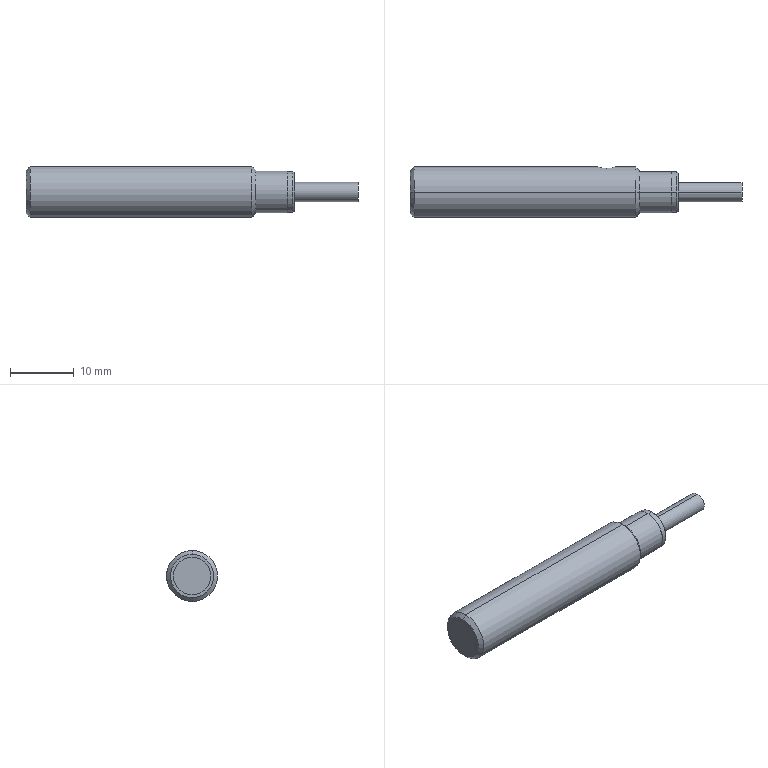Part | SolidWorks | features BaseBody 1 | 1 solid | 32 faces | box 52.05 x 8 x 8 mm | volume 2062 mm3 | cylinder 14 | plane 12 | cone 6 | commonest cylinder face diameters 3 x4 1.8 x2 5.9 x2 6.4 x2 6.5 x2 8 x2
STEP:
#1=CARTESIAN_POINT('',(30.8,3.708,-1.5));
#2=VERTEX_POINT('',#1);
#3=CARTESIAN_POINT('',(30.8,3.708,1.5));
#4=VERTEX_POINT('',#3);
#5=CARTESIAN_POINT('',(30.8,3.708,-1.5));
#6=CARTESIAN_POINT('',(30.997,3.708,-1.5));
#7=CARTESIAN_POINT('',(31.196,3.725,-1.46));
#8=CARTESIAN_POINT('',(31.467,3.767,-1.347));
#9=CARTESIAN_POINT('',(31.555,3.783,-1.3));
#10=CARTESIAN_POINT('',(31.717,3.819,-1.191));
#11=CARTESIAN_POINT('',(31.792,3.838,-1.13));
#12=CARTESIAN_POINT('',(31.999,3.895,-0.9226));
#13=CARTESIAN_POINT('',(32.109,3.932,-0.7596));
#14=CARTESIAN_POINT('',(32.223,3.972,-0.4853));
#15=CARTESIAN_POINT('',(32.251,3.982,-0.3914));
#16=CARTESIAN_POINT('',(32.29,3.996,-0.1986));
#17=CARTESIAN_POINT('',(32.3,4.,-0.09852));
#18=CARTESIAN_POINT('',(32.3,4.,0.09993));
#19=CARTESIAN_POINT('',(32.29,3.996,0.198));
#20=CARTESIAN_POINT('',(32.251,3.982,0.392));
#21=CARTESIAN_POINT('',(32.222,3.971,0.4877));
#22=CARTESIAN_POINT('',(32.109,3.932,0.7588));
#23=CARTESIAN_POINT('',(31.997,3.894,0.9245));
#24=CARTESIAN_POINT('',(31.791,3.838,1.13));
#25=CARTESIAN_POINT('',(31.715,3.818,1.193));
#26=CARTESIAN_POINT('',(31.553,3.783,1.301));
#27=CARTESIAN_POINT('',(31.467,3.767,1.347));
#28=CARTESIAN_POINT('',(31.286,3.739,1.423));
#29=CARTESIAN_POINT('',(31.19,3.727,1.452));
#30=CARTESIAN_POINT('',(30.997,3.712,1.49));
#31=CARTESIAN_POINT('',(30.9,3.708,1.5));
#32=CARTESIAN_POINT('',(30.8,3.708,1.5));
#33=B_SPLINE_CURVE_WITH_KNOTS('',3,(#5,#6,#7,#8,#9,#10,#11,#12,#13,#14,#15,#16,#17,#18,#19,#20,#21,#22,#23,#24,#25,#26,#27,#28,#29,#30,#31,#32),.UNSPECIFIED.,.F.,.F.,(4,2,2,2,2,2,2,2,2,2,2,2,2,4),(0.004683,0.005275,0.005571,0.005866,0.006458,0.006754,0.007049,0.007345,0.007641,0.008233,0.008528,0.008824,0.00912,0.009416),.UNSPECIFIED.);
#34=EDGE_CURVE('',#2,#4,#33,.T.);
#35=ORIENTED_EDGE('',*,*,#34,.T.);
#36=CARTESIAN_POINT('',(30.8,3.708,1.5));
#37=CARTESIAN_POINT('',(30.601,3.708,1.5));
#38=CARTESIAN_POINT('',(30.404,3.725,1.46));
#39=CARTESIAN_POINT('',(30.131,3.767,1.346));
#40=CARTESIAN_POINT('',(30.046,3.783,1.3));
#41=CARTESIAN_POINT('',(29.884,3.819,1.192));
#42=CARTESIAN_POINT('',(29.808,3.838,1.129));
#43=CARTESIAN_POINT('',(29.602,3.895,0.9231));
#44=CARTESIAN_POINT('',(29.491,3.932,0.7572));
#45=CARTESIAN_POINT('',(29.34,3.984,0.3969));
#46=CARTESIAN_POINT('',(29.3,4.,0.1979));
#47=CARTESIAN_POINT('',(29.3,4.,-0.0981));
#48=CARTESIAN_POINT('',(29.31,3.996,-0.1984));
#49=CARTESIAN_POINT('',(29.349,3.982,-0.3921));
#50=CARTESIAN_POINT('',(29.378,3.971,-0.486));
#51=CARTESIAN_POINT('',(29.491,3.932,-0.759));
#52=CARTESIAN_POINT('',(29.602,3.895,-0.9233));
#53=CARTESIAN_POINT('',(29.809,3.838,-1.13));
#54=CARTESIAN_POINT('',(29.884,3.819,-1.192));
#55=CARTESIAN_POINT('',(30.046,3.783,-1.3));
#56=CARTESIAN_POINT('',(30.133,3.767,-1.347));
#57=CARTESIAN_POINT('',(30.314,3.739,-1.422));
#58=CARTESIAN_POINT('',(30.407,3.728,-1.451));
#59=CARTESIAN_POINT('',(30.601,3.712,-1.49));
#60=CARTESIAN_POINT('',(30.701,3.708,-1.5));
#61=CARTESIAN_POINT('',(30.8,3.708,-1.5));
#62=B_SPLINE_CURVE_WITH_KNOTS('',3,(#36,#37,#38,#39,#40,#41,#42,#43,#44,#45,#46,#47,#48,#49,#50,#51,#52,#53,#54,#55,#56,#57,#58,#59,#60,#61),.UNSPECIFIED.,.F.,.F.,(4,2,2,2,2,2,2,2,2,2,2,2,4),(0.009416,0.01001,0.0103,0.0106,0.01119,0.01178,0.01208,0.01237,0.01296,0.01326,0.01356,0.01385,0.01415),.UNSPECIFIED.);
#63=EDGE_CURVE('',#4,#2,#62,.T.);
#64=ORIENTED_EDGE('',*,*,#63,.T.);
#65=EDGE_LOOP('',(#35,#64));
#66=FACE_BOUND('',#65,.T.);
#67=CARTESIAN_POINT('',(35.386,0.,4.));
#68=VERTEX_POINT('',#67);
#69=CARTESIAN_POINT('',(35.386,0.,-4.));
#70=VERTEX_POINT('',#69);
#71=CARTESIAN_POINT('',(35.386,0.,0.));
#72=DIRECTION('',(-1.,0.,0.));
#73=DIRECTION('',(0.,0.,1.));
#74=AXIS2_PLACEMENT_3D('',#71,#72,#73);
#75=CIRCLE('',#74,4.);
#76=EDGE_CURVE('',#68,#70,#75,.T.);
#77=ORIENTED_EDGE('',*,*,#76,.T.);
#78=CARTESIAN_POINT('',(0.6635,0.,-4.));
#79=VERTEX_POINT('',#78);
#80=CARTESIAN_POINT('',(52.05,0.,-4.));
#81=DIRECTION('',(-1.,0.,0.));
#82=VECTOR('',#81,1000.);
#83=LINE('',#80,#82);
#84=EDGE_CURVE('',#70,#79,#83,.T.);
#85=ORIENTED_EDGE('',*,*,#84,.T.);
#86=CARTESIAN_POINT('',(0.6635,0.,4.));
#87=VERTEX_POINT('',#86);
#88=CARTESIAN_POINT('',(0.6635,0.,0.));
#89=DIRECTION('',(1.,0.,0.));
#90=DIRECTION('',(0.,0.,1.));
#91=AXIS2_PLACEMENT_3D('',#88,#89,#90);
#92=CIRCLE('',#91,4.);
#93=EDGE_CURVE('',#79,#87,#92,.T.);
#94=ORIENTED_EDGE('',*,*,#93,.T.);
#95=CARTESIAN_POINT('',(52.05,0.,4.));
#96=DIRECTION('',(-1.,0.,0.));
#97=VECTOR('',#96,1000.);
#98=LINE('',#95,#97);
#99=EDGE_CURVE('',#68,#87,#98,.T.);
#100=ORIENTED_EDGE('',*,*,#99,.F.);
#101=EDGE_LOOP('',(#77,#85,#94,#100));
#102=FACE_OUTER_BOUND('',#101,.T.);
#103=CARTESIAN_POINT('',(52.05,0.,0.));
#104=DIRECTION('',(-1.,0.,0.));
#105=DIRECTION('',(0.,0.,1.));
#106=AXIS2_PLACEMENT_3D('',#103,#104,#105);
#107=CYLINDRICAL_SURFACE('',#106,4.);
#108=ADVANCED_FACE('',(#66,#102),#107,.T.);
#109=CARTESIAN_POINT('',(0.05,0.,-3.386));
#110=VERTEX_POINT('',#109);
#111=CARTESIAN_POINT('',(0.05,0.,3.386));
#112=VERTEX_POINT('',#111);
#113=CARTESIAN_POINT('',(0.05,0.,0.));
#114=DIRECTION('',(1.,0.,0.));
#115=DIRECTION('',(0.,0.,-1.));
#116=AXIS2_PLACEMENT_3D('',#113,#114,#115);
#117=CIRCLE('',#116,3.386);
#118=EDGE_CURVE('',#110,#112,#117,.T.);
#119=ORIENTED_EDGE('',*,*,#118,.T.);
#120=CARTESIAN_POINT('',(0.6635,0.,4.));
#121=DIRECTION('',(0.7071,0.,0.7071));
#122=VECTOR('',#121,1000.);
#123=LINE('',#120,#122);
#124=EDGE_CURVE('',#112,#87,#123,.T.);
#125=ORIENTED_EDGE('',*,*,#124,.T.);
#126=ORIENTED_EDGE('',*,*,#93,.F.);
#127=CARTESIAN_POINT('',(0.6635,0.,-4.));
#128=DIRECTION('',(0.7071,0.,-0.7071));
#129=VECTOR('',#128,1000.);
#130=LINE('',#127,#129);
#131=EDGE_CURVE('',#110,#79,#130,.T.);
#132=ORIENTED_EDGE('',*,*,#131,.F.);
#133=EDGE_LOOP('',(#119,#125,#126,#132));
#134=FACE_OUTER_BOUND('',#133,.T.);
#135=CARTESIAN_POINT('',(0.6635,0.,0.));
#136=DIRECTION('',(1.,0.,0.));
#137=DIRECTION('',(0.,0.,-1.));
#138=AXIS2_PLACEMENT_3D('',#135,#136,#137);
#139=CONICAL_SURFACE('',#138,4.,0.7854);
#140=ADVANCED_FACE('',(#134),#139,.T.);
#141=ORIENTED_EDGE('',*,*,#63,.F.);
#142=CARTESIAN_POINT('',(30.8,2.75,1.5));
#143=VERTEX_POINT('',#142);
#144=CARTESIAN_POINT('',(30.8,2.75,1.5));
#145=DIRECTION('',(0.,-1.,0.));
#146=VECTOR('',#145,1000.);
#147=LINE('',#144,#146);
#148=EDGE_CURVE('',#4,#143,#147,.T.);
#149=ORIENTED_EDGE('',*,*,#148,.T.);
#150=CARTESIAN_POINT('',(30.8,2.75,-1.5));
#151=VERTEX_POINT('',#150);
#152=CARTESIAN_POINT('',(30.8,2.75,0.));
#153=DIRECTION('',(0.,1.,0.));
#154=DIRECTION('',(0.,0.,-1.));
#155=AXIS2_PLACEMENT_3D('',#152,#153,#154);
#156=CIRCLE('',#155,1.5);
#157=EDGE_CURVE('',#151,#143,#156,.T.);
#158=ORIENTED_EDGE('',*,*,#157,.F.);
#159=CARTESIAN_POINT('',(30.8,2.75,-1.5));
#160=DIRECTION('',(0.,-1.,0.));
#161=VECTOR('',#160,1000.);
#162=LINE('',#159,#161);
#163=EDGE_CURVE('',#2,#151,#162,.T.);
#164=ORIENTED_EDGE('',*,*,#163,.F.);
#165=EDGE_LOOP('',(#141,#149,#158,#164));
#166=FACE_OUTER_BOUND('',#165,.T.);
#167=CARTESIAN_POINT('',(30.8,2.75,0.));
#168=DIRECTION('',(0.,-1.,0.));
#169=DIRECTION('',(0.,0.,-1.));
#170=AXIS2_PLACEMENT_3D('',#167,#168,#169);
#171=CYLINDRICAL_SURFACE('',#170,1.5);
#172=ADVANCED_FACE('',(#166),#171,.F.);
#173=CARTESIAN_POINT('',(36.,0.,3.387));
#174=VERTEX_POINT('',#173);
#175=CARTESIAN_POINT('',(36.,0.,-3.387));
#176=VERTEX_POINT('',#175);
#177=CARTESIAN_POINT('',(36.,0.,0.));
#178=DIRECTION('',(-1.,0.,0.));
#179=DIRECTION('',(0.,0.,1.));
#180=AXIS2_PLACEMENT_3D('',#177,#178,#179);
#181=CIRCLE('',#180,3.387);
#182=EDGE_CURVE('',#174,#176,#181,.T.);
#183=ORIENTED_EDGE('',*,*,#182,.T.);
#184=CARTESIAN_POINT('',(35.387,0.,-4.));
#185=DIRECTION('',(-0.7071,0.,-0.7071));
#186=VECTOR('',#185,1000.);
#187=LINE('',#184,#186);
#188=EDGE_CURVE('',#176,#70,#187,.T.);
#189=ORIENTED_EDGE('',*,*,#188,.T.);
#190=ORIENTED_EDGE('',*,*,#76,.F.);
#191=CARTESIAN_POINT('',(35.387,0.,4.));
#192=DIRECTION('',(-0.7071,0.,0.7071));
#193=VECTOR('',#192,1000.);
#194=LINE('',#191,#193);
#195=EDGE_CURVE('',#174,#68,#194,.T.);
#196=ORIENTED_EDGE('',*,*,#195,.F.);
#197=EDGE_LOOP('',(#183,#189,#190,#196));
#198=FACE_OUTER_BOUND('',#197,.T.);
#199=CARTESIAN_POINT('',(35.387,0.,0.));
#200=DIRECTION('',(-1.,0.,0.));
#201=DIRECTION('',(0.,0.,1.));
#202=AXIS2_PLACEMENT_3D('',#199,#200,#201);
#203=CONICAL_SURFACE('',#202,4.,0.7854);
#204=ADVANCED_FACE('',(#198),#203,.T.);
#205=CARTESIAN_POINT('',(0.05,0.,2.95));
#206=VERTEX_POINT('',#205);
#207=CARTESIAN_POINT('',(0.05,0.,-2.95));
#208=VERTEX_POINT('',#207);
#209=CARTESIAN_POINT('',(0.05,0.,0.));
#210=DIRECTION('',(-1.,0.,0.));
#211=DIRECTION('',(0.,0.,1.));
#212=AXIS2_PLACEMENT_3D('',#209,#210,#211);
#213=CIRCLE('',#212,2.95);
#214=EDGE_CURVE('',#206,#208,#213,.T.);
#215=ORIENTED_EDGE('',*,*,#214,.T.);
#216=CARTESIAN_POINT('',(0.,0.,-2.95));
#217=VERTEX_POINT('',#216);
#218=CARTESIAN_POINT('',(52.05,0.,-2.95));
#219=DIRECTION('',(-1.,0.,0.));
#220=VECTOR('',#219,1000.);
#221=LINE('',#218,#220);
#222=EDGE_CURVE('',#208,#217,#221,.T.);
#223=ORIENTED_EDGE('',*,*,#222,.T.);
#224=CARTESIAN_POINT('',(0.,0.,2.95));
#225=VERTEX_POINT('',#224);
#226=CARTESIAN_POINT('',(0.,0.,0.));
#227=DIRECTION('',(1.,0.,0.));
#228=DIRECTION('',(0.,0.,1.));
#229=AXIS2_PLACEMENT_3D('',#226,#227,#228);
#230=CIRCLE('',#229,2.95);
#231=EDGE_CURVE('',#217,#225,#230,.T.);
#232=ORIENTED_EDGE('',*,*,#231,.T.);
#233=CARTESIAN_POINT('',(52.05,0.,2.95));
#234=DIRECTION('',(-1.,0.,0.));
#235=VECTOR('',#234,1000.);
#236=LINE('',#233,#235);
#237=EDGE_CURVE('',#206,#225,#236,.T.);
#238=ORIENTED_EDGE('',*,*,#237,.F.);
#239=EDGE_LOOP('',(#215,#223,#232,#238));
#240=FACE_OUTER_BOUND('',#239,.T.);
#241=CARTESIAN_POINT('',(52.05,0.,0.));
#242=DIRECTION('',(-1.,0.,0.));
#243=DIRECTION('',(0.,0.,1.));
#244=AXIS2_PLACEMENT_3D('',#241,#242,#243);
#245=CYLINDRICAL_SURFACE('',#244,2.95);
#246=ADVANCED_FACE('',(#240),#245,.T.);
#247=CARTESIAN_POINT('',(30.8,2.9,0.9));
#248=VERTEX_POINT('',#247);
#249=CARTESIAN_POINT('',(31.05,2.9,0.8646));
#250=VERTEX_POINT('',#249);
#251=CARTESIAN_POINT('',(30.8,2.9,0.));
#252=DIRECTION('',(0.,1.,0.));
#253=DIRECTION('',(0.,0.,-1.));
#254=AXIS2_PLACEMENT_3D('',#251,#252,#253);
#255=CIRCLE('',#254,0.9);
#256=EDGE_CURVE('',#248,#250,#255,.T.);
#257=ORIENTED_EDGE('',*,*,#256,.F.);
#258=CARTESIAN_POINT('',(30.8,2.75,0.9));
#259=VERTEX_POINT('',#258);
#260=CARTESIAN_POINT('',(30.8,2.55,0.9));
#261=DIRECTION('',(0.,-1.,0.));
#262=VECTOR('',#261,1000.);
#263=LINE('',#260,#262);
#264=EDGE_CURVE('',#248,#259,#263,.T.);
#265=ORIENTED_EDGE('',*,*,#264,.T.);
#266=CARTESIAN_POINT('',(30.8,2.75,-0.9));
#267=VERTEX_POINT('',#266);
#268=CARTESIAN_POINT('',(30.8,2.75,0.));
#269=DIRECTION('',(0.,-1.,0.));
#270=DIRECTION('',(0.,0.,-1.));
#271=AXIS2_PLACEMENT_3D('',#268,#269,#270);
#272=CIRCLE('',#271,0.9);
#273=EDGE_CURVE('',#267,#259,#272,.T.);
#274=ORIENTED_EDGE('',*,*,#273,.F.);
#275=CARTESIAN_POINT('',(30.8,2.9,-0.9));
#276=VERTEX_POINT('',#275);
#277=CARTESIAN_POINT('',(30.8,2.55,-0.9));
#278=DIRECTION('',(0.,-1.,0.));
#279=VECTOR('',#278,1000.);
#280=LINE('',#277,#279);
#281=EDGE_CURVE('',#276,#267,#280,.T.);
#282=ORIENTED_EDGE('',*,*,#281,.F.);
#283=CARTESIAN_POINT('',(31.05,2.9,-0.8646));
#284=VERTEX_POINT('',#283);
#285=CARTESIAN_POINT('',(30.8,2.9,0.));
#286=DIRECTION('',(0.,1.,0.));
#287=DIRECTION('',(0.,0.,-1.));
#288=AXIS2_PLACEMENT_3D('',#285,#286,#287);
#289=CIRCLE('',#288,0.9);
#290=EDGE_CURVE('',#284,#276,#289,.T.);
#291=ORIENTED_EDGE('',*,*,#290,.F.);
#292=CARTESIAN_POINT('',(31.05,3.05,-0.8646));
#293=VERTEX_POINT('',#292);
#294=CARTESIAN_POINT('',(31.05,2.9,-0.8646));
#295=DIRECTION('',(0.,1.,0.));
#296=VECTOR('',#295,1000.);
#297=LINE('',#294,#296);
#298=EDGE_CURVE('',#284,#293,#297,.T.);
#299=ORIENTED_EDGE('',*,*,#298,.T.);
#300=CARTESIAN_POINT('',(31.05,3.05,0.8646));
#301=VERTEX_POINT('',#300);
#302=CARTESIAN_POINT('',(30.8,3.05,0.));
#303=DIRECTION('',(0.,-1.,0.));
#304=DIRECTION('',(0.,0.,-1.));
#305=AXIS2_PLACEMENT_3D('',#302,#303,#304);
#306=CIRCLE('',#305,0.9);
#307=EDGE_CURVE('',#293,#301,#306,.T.);
#308=ORIENTED_EDGE('',*,*,#307,.T.);
#309=CARTESIAN_POINT('',(31.05,2.9,0.8646));
#310=DIRECTION('',(0.,-1.,0.));
#311=VECTOR('',#310,1000.);
#312=LINE('',#309,#311);
#313=EDGE_CURVE('',#301,#250,#312,.T.);
#314=ORIENTED_EDGE('',*,*,#313,.T.);
#315=EDGE_LOOP('',(#257,#265,#274,#282,#291,#299,#308,#314));
#316=FACE_OUTER_BOUND('',#315,.T.);
#317=CARTESIAN_POINT('',(30.8,2.55,0.));
#318=DIRECTION('',(0.,-1.,0.));
#319=DIRECTION('',(0.,0.,-1.));
#320=AXIS2_PLACEMENT_3D('',#317,#318,#319);
#321=CYLINDRICAL_SURFACE('',#320,0.9);
#322=ADVANCED_FACE('',(#316),#321,.T.);
#323=CARTESIAN_POINT('',(41.05,0.,3.25));
#324=VERTEX_POINT('',#323);
#325=CARTESIAN_POINT('',(41.05,0.,-3.25));
#326=VERTEX_POINT('',#325);
#327=CARTESIAN_POINT('',(41.05,0.,0.));
#328=DIRECTION('',(-1.,0.,0.));
#329=DIRECTION('',(0.,0.,1.));
#330=AXIS2_PLACEMENT_3D('',#327,#328,#329);
#331=CIRCLE('',#330,3.25);
#332=EDGE_CURVE('',#324,#326,#331,.T.);
#333=ORIENTED_EDGE('',*,*,#332,.T.);
#334=CARTESIAN_POINT('',(36.,0.,-3.25));
#335=VERTEX_POINT('',#334);
#336=CARTESIAN_POINT('',(52.05,0.,-3.25));
#337=DIRECTION('',(-1.,0.,0.));
#338=VECTOR('',#337,1000.);
#339=LINE('',#336,#338);
#340=EDGE_CURVE('',#326,#335,#339,.T.);
#341=ORIENTED_EDGE('',*,*,#340,.T.);
#342=CARTESIAN_POINT('',(36.,0.,3.25));
#343=VERTEX_POINT('',#342);
#344=CARTESIAN_POINT('',(36.,0.,0.));
#345=DIRECTION('',(1.,0.,0.));
#346=DIRECTION('',(0.,0.,1.));
#347=AXIS2_PLACEMENT_3D('',#344,#345,#346);
#348=CIRCLE('',#347,3.25);
#349=EDGE_CURVE('',#335,#343,#348,.T.);
#350=ORIENTED_EDGE('',*,*,#349,.T.);
#351=CARTESIAN_POINT('',(52.05,0.,3.25));
#352=DIRECTION('',(-1.,0.,0.));
#353=VECTOR('',#352,1000.);
#354=LINE('',#351,#353);
#355=EDGE_CURVE('',#324,#343,#354,.T.);
#356=ORIENTED_EDGE('',*,*,#355,.F.);
#357=EDGE_LOOP('',(#333,#341,#350,#356));
#358=FACE_OUTER_BOUND('',#357,.T.);
#359=CARTESIAN_POINT('',(52.05,0.,0.));
#360=DIRECTION('',(-1.,0.,0.));
#361=DIRECTION('',(0.,0.,1.));
#362=AXIS2_PLACEMENT_3D('',#359,#360,#361);
#363=CYLINDRICAL_SURFACE('',#362,3.25);
#364=ADVANCED_FACE('',(#358),#363,.T.);
#365=CARTESIAN_POINT('',(41.85,0.,3.2));
#366=VERTEX_POINT('',#365);
#367=CARTESIAN_POINT('',(41.85,0.,-3.2));
#368=VERTEX_POINT('',#367);
#369=CARTESIAN_POINT('',(41.85,0.,0.));
#370=DIRECTION('',(-1.,0.,0.));
#371=DIRECTION('',(0.,0.,1.));
#372=AXIS2_PLACEMENT_3D('',#369,#370,#371);
#373=CIRCLE('',#372,3.2);
#374=EDGE_CURVE('',#366,#368,#373,.T.);
#375=ORIENTED_EDGE('',*,*,#374,.T.);
#376=CARTESIAN_POINT('',(41.05,0.,-3.2));
#377=VERTEX_POINT('',#376);
#378=CARTESIAN_POINT('',(52.05,0.,-3.2));
#379=DIRECTION('',(-1.,0.,0.));
#380=VECTOR('',#379,1000.);
#381=LINE('',#378,#380);
#382=EDGE_CURVE('',#368,#377,#381,.T.);
#383=ORIENTED_EDGE('',*,*,#382,.T.);
#384=CARTESIAN_POINT('',(41.05,0.,3.2));
#385=VERTEX_POINT('',#384);
#386=CARTESIAN_POINT('',(41.05,0.,0.));
#387=DIRECTION('',(1.,0.,0.));
#388=DIRECTION('',(0.,0.,1.));
#389=AXIS2_PLACEMENT_3D('',#386,#387,#388);
#390=CIRCLE('',#389,3.2);
#391=EDGE_CURVE('',#377,#385,#390,.T.);
#392=ORIENTED_EDGE('',*,*,#391,.T.);
#393=CARTESIAN_POINT('',(52.05,0.,3.2));
#394=DIRECTION('',(-1.,0.,0.));
#395=VECTOR('',#394,1000.);
#396=LINE('',#393,#395);
#397=EDGE_CURVE('',#366,#385,#396,.T.);
#398=ORIENTED_EDGE('',*,*,#397,.F.);
#399=EDGE_LOOP('',(#375,#383,#392,#398));
#400=FACE_OUTER_BOUND('',#399,.T.);
#401=CARTESIAN_POINT('',(52.05,0.,0.));
#402=DIRECTION('',(-1.,0.,0.));
#403=DIRECTION('',(0.,0.,1.));
#404=AXIS2_PLACEMENT_3D('',#401,#402,#403);
#405=CYLINDRICAL_SURFACE('',#404,3.2);
#406=ADVANCED_FACE('',(#400),#405,.T.);
#407=CARTESIAN_POINT('',(42.05,0.,3.));
#408=VERTEX_POINT('',#407);
#409=CARTESIAN_POINT('',(42.05,0.,-3.));
#410=VERTEX_POINT('',#409);
#411=CARTESIAN_POINT('',(42.05,0.,0.));
#412=DIRECTION('',(-1.,0.,0.));
#413=DIRECTION('',(0.,0.,1.));
#414=AXIS2_PLACEMENT_3D('',#411,#412,#413);
#415=CIRCLE('',#414,3.);
#416=EDGE_CURVE('',#408,#410,#415,.T.);
#417=ORIENTED_EDGE('',*,*,#416,.T.);
#418=CARTESIAN_POINT('',(41.85,0.,-3.2));
#419=DIRECTION('',(-0.7071,0.,-0.7071));
#420=VECTOR('',#419,1000.);
#421=LINE('',#418,#420);
#422=EDGE_CURVE('',#410,#368,#421,.T.);
#423=ORIENTED_EDGE('',*,*,#422,.T.);
#424=ORIENTED_EDGE('',*,*,#374,.F.);
#425=CARTESIAN_POINT('',(41.85,0.,3.2));
#426=DIRECTION('',(-0.7071,0.,0.7071));
#427=VECTOR('',#426,1000.);
#428=LINE('',#425,#427);
#429=EDGE_CURVE('',#408,#366,#428,.T.);
#430=ORIENTED_EDGE('',*,*,#429,.F.);
#431=EDGE_LOOP('',(#417,#423,#424,#430));
#432=FACE_OUTER_BOUND('',#431,.T.);
#433=CARTESIAN_POINT('',(41.85,0.,0.));
#434=DIRECTION('',(-1.,0.,0.));
#435=DIRECTION('',(0.,0.,1.));
#436=AXIS2_PLACEMENT_3D('',#433,#434,#435);
#437=CONICAL_SURFACE('',#436,3.2,0.7854);
#438=ADVANCED_FACE('',(#432),#437,.T.);
#439=CARTESIAN_POINT('',(52.05,0.,1.5));
#440=VERTEX_POINT('',#439);
#441=CARTESIAN_POINT('',(52.05,0.,-1.5));
#442=VERTEX_POINT('',#441);
#443=CARTESIAN_POINT('',(52.05,0.,0.));
#444=DIRECTION('',(-1.,0.,0.));
#445=DIRECTION('',(0.,0.,1.));
#446=AXIS2_PLACEMENT_3D('',#443,#444,#445);
#447=CIRCLE('',#446,1.5);
#448=EDGE_CURVE('',#440,#442,#447,.T.);
#449=ORIENTED_EDGE('',*,*,#448,.T.);
#450=CARTESIAN_POINT('',(42.05,0.,-1.5));
#451=VERTEX_POINT('',#450);
#452=CARTESIAN_POINT('',(52.05,0.,-1.5));
#453=DIRECTION('',(-1.,0.,0.));
#454=VECTOR('',#453,1000.);
#455=LINE('',#452,#454);
#456=EDGE_CURVE('',#442,#451,#455,.T.);
#457=ORIENTED_EDGE('',*,*,#456,.T.);
#458=CARTESIAN_POINT('',(42.05,0.,1.5));
#459=VERTEX_POINT('',#458);
#460=CARTESIAN_POINT('',(42.05,0.,0.));
#461=DIRECTION('',(1.,0.,0.));
#462=DIRECTION('',(0.,0.,1.));
#463=AXIS2_PLACEMENT_3D('',#460,#461,#462);
#464=CIRCLE('',#463,1.5);
#465=EDGE_CURVE('',#451,#459,#464,.T.);
#466=ORIENTED_EDGE('',*,*,#465,.T.);
#467=CARTESIAN_POINT('',(52.05,0.,1.5));
#468=DIRECTION('',(-1.,0.,0.));
#469=VECTOR('',#468,1000.);
#470=LINE('',#467,#469);
#471=EDGE_CURVE('',#440,#459,#470,.T.);
#472=ORIENTED_EDGE('',*,*,#471,.F.);
#473=EDGE_LOOP('',(#449,#457,#466,#472));
#474=FACE_OUTER_BOUND('',#473,.T.);
#475=CARTESIAN_POINT('',(52.05,0.,0.));
#476=DIRECTION('',(-1.,0.,0.));
#477=DIRECTION('',(0.,0.,1.));
#478=AXIS2_PLACEMENT_3D('',#475,#476,#477);
#479=CYLINDRICAL_SURFACE('',#478,1.5);
#480=ADVANCED_FACE('',(#474),#479,.T.);
#481=ORIENTED_EDGE('',*,*,#84,.F.);
#482=CARTESIAN_POINT('',(35.386,0.,0.));
#483=DIRECTION('',(-1.,0.,0.));
#484=DIRECTION('',(0.,0.,1.));
#485=AXIS2_PLACEMENT_3D('',#482,#483,#484);
#486=CIRCLE('',#485,4.);
#487=EDGE_CURVE('',#70,#68,#486,.T.);
#488=ORIENTED_EDGE('',*,*,#487,.T.);
#489=ORIENTED_EDGE('',*,*,#99,.T.);
#490=CARTESIAN_POINT('',(0.6635,0.,0.));
#491=DIRECTION('',(1.,0.,0.));
#492=DIRECTION('',(0.,0.,1.));
#493=AXIS2_PLACEMENT_3D('',#490,#491,#492);
#494=CIRCLE('',#493,4.);
#495=EDGE_CURVE('',#87,#79,#494,.T.);
#496=ORIENTED_EDGE('',*,*,#495,.T.);
#497=EDGE_LOOP('',(#481,#488,#489,#496));
#498=FACE_OUTER_BOUND('',#497,.T.);
#499=CARTESIAN_POINT('',(52.05,0.,0.));
#500=DIRECTION('',(-1.,0.,0.));
#501=DIRECTION('',(0.,0.,1.));
#502=AXIS2_PLACEMENT_3D('',#499,#500,#501);
#503=CYLINDRICAL_SURFACE('',#502,4.);
#504=ADVANCED_FACE('',(#498),#503,.T.);
#505=ORIENTED_EDGE('',*,*,#124,.F.);
#506=CARTESIAN_POINT('',(0.05,0.,0.));
#507=DIRECTION('',(1.,0.,0.));
#508=DIRECTION('',(0.,0.,-1.));
#509=AXIS2_PLACEMENT_3D('',#506,#507,#508);
#510=CIRCLE('',#509,3.386);
#511=EDGE_CURVE('',#112,#110,#510,.T.);
#512=ORIENTED_EDGE('',*,*,#511,.T.);
#513=ORIENTED_EDGE('',*,*,#131,.T.);
#514=ORIENTED_EDGE('',*,*,#495,.F.);
#515=EDGE_LOOP('',(#505,#512,#513,#514));
#516=FACE_OUTER_BOUND('',#515,.T.);
#517=CARTESIAN_POINT('',(0.6635,0.,0.));
#518=DIRECTION('',(1.,0.,0.));
#519=DIRECTION('',(0.,0.,-1.));
#520=AXIS2_PLACEMENT_3D('',#517,#518,#519);
#521=CONICAL_SURFACE('',#520,4.,0.7854);
#522=ADVANCED_FACE('',(#516),#521,.T.);
#523=ORIENTED_EDGE('',*,*,#148,.F.);
#524=ORIENTED_EDGE('',*,*,#34,.F.);
#525=ORIENTED_EDGE('',*,*,#163,.T.);
#526=CARTESIAN_POINT('',(30.8,2.75,0.));
#527=DIRECTION('',(0.,1.,0.));
#528=DIRECTION('',(0.,0.,-1.));
#529=AXIS2_PLACEMENT_3D('',#526,#527,#528);
#530=CIRCLE('',#529,1.5);
#531=EDGE_CURVE('',#143,#151,#530,.T.);
#532=ORIENTED_EDGE('',*,*,#531,.F.);
#533=EDGE_LOOP('',(#523,#524,#525,#532));
#534=FACE_OUTER_BOUND('',#533,.T.);
#535=CARTESIAN_POINT('',(30.8,2.75,0.));
#536=DIRECTION('',(0.,-1.,0.));
#537=DIRECTION('',(0.,0.,-1.));
#538=AXIS2_PLACEMENT_3D('',#535,#536,#537);
#539=CYLINDRICAL_SURFACE('',#538,1.5);
#540=ADVANCED_FACE('',(#534),#539,.F.);
#541=ORIENTED_EDGE('',*,*,#188,.F.);
#542=CARTESIAN_POINT('',(36.,0.,0.));
#543=DIRECTION('',(-1.,0.,0.));
#544=DIRECTION('',(0.,0.,1.));
#545=AXIS2_PLACEMENT_3D('',#542,#543,#544);
#546=CIRCLE('',#545,3.387);
#547=EDGE_CURVE('',#176,#174,#546,.T.);
#548=ORIENTED_EDGE('',*,*,#547,.T.);
#549=ORIENTED_EDGE('',*,*,#195,.T.);
#550=ORIENTED_EDGE('',*,*,#487,.F.);
#551=EDGE_LOOP('',(#541,#548,#549,#550));
#552=FACE_OUTER_BOUND('',#551,.T.);
#553=CARTESIAN_POINT('',(35.387,0.,0.));
#554=DIRECTION('',(-1.,0.,0.));
#555=DIRECTION('',(0.,0.,1.));
#556=AXIS2_PLACEMENT_3D('',#553,#554,#555);
#557=CONICAL_SURFACE('',#556,4.,0.7854);
#558=ADVANCED_FACE('',(#552),#557,.T.);
#559=ORIENTED_EDGE('',*,*,#214,.F.);
#560=CARTESIAN_POINT('',(0.05,0.,0.));
#561=DIRECTION('',(-1.,0.,0.));
#562=DIRECTION('',(0.,0.,1.));
#563=AXIS2_PLACEMENT_3D('',#560,#561,#562);
#564=CIRCLE('',#563,2.95);
#565=EDGE_CURVE('',#208,#206,#564,.T.);
#566=ORIENTED_EDGE('',*,*,#565,.F.);
#567=EDGE_LOOP('',(#559,#566));
#568=FACE_BOUND('',#567,.T.);
#569=ORIENTED_EDGE('',*,*,#118,.F.);
#570=ORIENTED_EDGE('',*,*,#511,.F.);
#571=EDGE_LOOP('',(#569,#570));
#572=FACE_OUTER_BOUND('',#571,.T.);
#573=CARTESIAN_POINT('',(0.05,2.95,0.));
#574=DIRECTION('',(1.,0.,0.));
#575=DIRECTION('',(0.,0.,-1.));
#576=AXIS2_PLACEMENT_3D('',#573,#574,#575);
#577=PLANE('',#576);
#578=ADVANCED_FACE('',(#568,#572),#577,.F.);
#579=ORIENTED_EDGE('',*,*,#157,.T.);
#580=ORIENTED_EDGE('',*,*,#531,.T.);
#581=EDGE_LOOP('',(#579,#580));
#582=FACE_OUTER_BOUND('',#581,.T.);
#583=ORIENTED_EDGE('',*,*,#273,.T.);
#584=CARTESIAN_POINT('',(30.8,2.75,0.));
#585=DIRECTION('',(0.,-1.,0.));
#586=DIRECTION('',(0.,0.,-1.));
#587=AXIS2_PLACEMENT_3D('',#584,#585,#586);
#588=CIRCLE('',#587,0.9);
#589=EDGE_CURVE('',#259,#267,#588,.T.);
#590=ORIENTED_EDGE('',*,*,#589,.T.);
#591=EDGE_LOOP('',(#583,#590));
#592=FACE_BOUND('',#591,.T.);
#593=CARTESIAN_POINT('',(30.8,2.75,0.));
#594=DIRECTION('',(0.,1.,0.));
#595=DIRECTION('',(0.,0.,1.));
#596=AXIS2_PLACEMENT_3D('',#593,#594,#595);
#597=PLANE('',#596);
#598=ADVANCED_FACE('',(#582,#592),#597,.T.);
#599=ORIENTED_EDGE('',*,*,#182,.F.);
#600=ORIENTED_EDGE('',*,*,#547,.F.);
#601=EDGE_LOOP('',(#599,#600));
#602=FACE_OUTER_BOUND('',#601,.T.);
#603=CARTESIAN_POINT('',(36.,0.,0.));
#604=DIRECTION('',(1.,0.,0.));
#605=DIRECTION('',(0.,0.,1.));
#606=AXIS2_PLACEMENT_3D('',#603,#604,#605);
#607=CIRCLE('',#606,3.25);
#608=EDGE_CURVE('',#343,#335,#607,.T.);
#609=ORIENTED_EDGE('',*,*,#608,.F.);
#610=ORIENTED_EDGE('',*,*,#349,.F.);
#611=EDGE_LOOP('',(#609,#610));
#612=FACE_BOUND('',#611,.T.);
#613=CARTESIAN_POINT('',(36.,3.386,0.));
#614=DIRECTION('',(-1.,0.,0.));
#615=DIRECTION('',(0.,0.,1.));
#616=AXIS2_PLACEMENT_3D('',#613,#614,#615);
#617=PLANE('',#616);
#618=ADVANCED_FACE('',(#602,#612),#617,.F.);
#619=ORIENTED_EDGE('',*,*,#222,.F.);
#620=ORIENTED_EDGE('',*,*,#565,.T.);
#621=ORIENTED_EDGE('',*,*,#237,.T.);
#622=CARTESIAN_POINT('',(0.,0.,0.));
#623=DIRECTION('',(1.,0.,0.));
#624=DIRECTION('',(0.,0.,1.));
#625=AXIS2_PLACEMENT_3D('',#622,#623,#624);
#626=CIRCLE('',#625,2.95);
#627=EDGE_CURVE('',#225,#217,#626,.T.);
#628=ORIENTED_EDGE('',*,*,#627,.T.);
#629=EDGE_LOOP('',(#619,#620,#621,#628));
#630=FACE_OUTER_BOUND('',#629,.T.);
#631=CARTESIAN_POINT('',(52.05,0.,0.));
#632=DIRECTION('',(-1.,0.,0.));
#633=DIRECTION('',(0.,0.,1.));
#634=AXIS2_PLACEMENT_3D('',#631,#632,#633);
#635=CYLINDRICAL_SURFACE('',#634,2.95);
#636=ADVANCED_FACE('',(#630),#635,.T.);
#637=ORIENTED_EDGE('',*,*,#264,.F.);
#638=CARTESIAN_POINT('',(30.55,2.9,0.8646));
#639=VERTEX_POINT('',#638);
#640=CARTESIAN_POINT('',(30.8,2.9,0.));
#641=DIRECTION('',(0.,1.,0.));
#642=DIRECTION('',(0.,0.,-1.));
#643=AXIS2_PLACEMENT_3D('',#640,#641,#642);
#644=CIRCLE('',#643,0.9);
#645=EDGE_CURVE('',#639,#248,#644,.T.);
#646=ORIENTED_EDGE('',*,*,#645,.F.);
#647=CARTESIAN_POINT('',(30.55,3.05,0.8646));
#648=VERTEX_POINT('',#647);
#649=CARTESIAN_POINT('',(30.55,2.9,0.8646));
#650=DIRECTION('',(0.,1.,0.));
#651=VECTOR('',#650,1000.);
#652=LINE('',#649,#651);
#653=EDGE_CURVE('',#639,#648,#652,.T.);
#654=ORIENTED_EDGE('',*,*,#653,.T.);
#655=CARTESIAN_POINT('',(30.55,3.05,-0.8646));
#656=VERTEX_POINT('',#655);
#657=CARTESIAN_POINT('',(30.8,3.05,0.));
#658=DIRECTION('',(0.,-1.,0.));
#659=DIRECTION('',(0.,0.,-1.));
#660=AXIS2_PLACEMENT_3D('',#657,#658,#659);
#661=CIRCLE('',#660,0.9);
#662=EDGE_CURVE('',#648,#656,#661,.T.);
#663=ORIENTED_EDGE('',*,*,#662,.T.);
#664=CARTESIAN_POINT('',(30.55,2.9,-0.8646));
#665=VERTEX_POINT('',#664);
#666=CARTESIAN_POINT('',(30.55,2.9,-0.8646));
#667=DIRECTION('',(0.,-1.,0.));
#668=VECTOR('',#667,1000.);
#669=LINE('',#666,#668);
#670=EDGE_CURVE('',#656,#665,#669,.T.);
#671=ORIENTED_EDGE('',*,*,#670,.T.);
#672=CARTESIAN_POINT('',(30.8,2.9,0.));
#673=DIRECTION('',(0.,1.,0.));
#674=DIRECTION('',(0.,0.,-1.));
#675=AXIS2_PLACEMENT_3D('',#672,#673,#674);
#676=CIRCLE('',#675,0.9);
#677=EDGE_CURVE('',#276,#665,#676,.T.);
#678=ORIENTED_EDGE('',*,*,#677,.F.);
#679=ORIENTED_EDGE('',*,*,#281,.T.);
#680=ORIENTED_EDGE('',*,*,#589,.F.);
#681=EDGE_LOOP('',(#637,#646,#654,#663,#671,#678,#679,#680));
#682=FACE_OUTER_BOUND('',#681,.T.);
#683=CARTESIAN_POINT('',(30.8,2.55,0.));
#684=DIRECTION('',(0.,-1.,0.));
#685=DIRECTION('',(0.,0.,-1.));
#686=AXIS2_PLACEMENT_3D('',#683,#684,#685);
#687=CYLINDRICAL_SURFACE('',#686,0.9);
#688=ADVANCED_FACE('',(#682),#687,.T.);
#689=ORIENTED_EDGE('',*,*,#340,.F.);
#690=CARTESIAN_POINT('',(41.05,0.,0.));
#691=DIRECTION('',(-1.,0.,0.));
#692=DIRECTION('',(0.,0.,1.));
#693=AXIS2_PLACEMENT_3D('',#690,#691,#692);
#694=CIRCLE('',#693,3.25);
#695=EDGE_CURVE('',#326,#324,#694,.T.);
#696=ORIENTED_EDGE('',*,*,#695,.T.);
#697=ORIENTED_EDGE('',*,*,#355,.T.);
#698=ORIENTED_EDGE('',*,*,#608,.T.);
#699=EDGE_LOOP('',(#689,#696,#697,#698));
#700=FACE_OUTER_BOUND('',#699,.T.);
#701=CARTESIAN_POINT('',(52.05,0.,0.));
#702=DIRECTION('',(-1.,0.,0.));
#703=DIRECTION('',(0.,0.,1.));
#704=AXIS2_PLACEMENT_3D('',#701,#702,#703);
#705=CYLINDRICAL_SURFACE('',#704,3.25);
#706=ADVANCED_FACE('',(#700),#705,.T.);
#707=ORIENTED_EDGE('',*,*,#627,.F.);
#708=ORIENTED_EDGE('',*,*,#231,.F.);
#709=EDGE_LOOP('',(#707,#708));
#710=FACE_OUTER_BOUND('',#709,.T.);
#711=CARTESIAN_POINT('',(0.,0.,0.));
#712=DIRECTION('',(1.,0.,0.));
#713=DIRECTION('',(0.,0.,-1.));
#714=AXIS2_PLACEMENT_3D('',#711,#712,#713);
#715=PLANE('',#714);
#716=ADVANCED_FACE('',(#710),#715,.F.);
#717=CARTESIAN_POINT('',(30.55,3.05,0.));
#718=DIRECTION('',(0.,0.,-1.));
#719=VECTOR('',#718,1000.);
#720=LINE('',#717,#719);
#721=EDGE_CURVE('',#648,#656,#720,.T.);
#722=ORIENTED_EDGE('',*,*,#721,.T.);
#723=ORIENTED_EDGE('',*,*,#662,.F.);
#724=EDGE_LOOP('',(#722,#723));
#725=FACE_OUTER_BOUND('',#724,.T.);
#726=CARTESIAN_POINT('',(30.8,3.05,0.));
#727=DIRECTION('',(0.,1.,0.));
#728=DIRECTION('',(0.,0.,1.));
#729=AXIS2_PLACEMENT_3D('',#726,#727,#728);
#730=PLANE('',#729);
#731=ADVANCED_FACE('',(#725),#730,.T.);
#732=CARTESIAN_POINT('',(31.05,3.05,0.));
#733=DIRECTION('',(0.,0.,1.));
#734=VECTOR('',#733,1000.);
#735=LINE('',#732,#734);
#736=EDGE_CURVE('',#293,#301,#735,.T.);
#737=ORIENTED_EDGE('',*,*,#736,.T.);
#738=ORIENTED_EDGE('',*,*,#307,.F.);
#739=EDGE_LOOP('',(#737,#738));
#740=FACE_OUTER_BOUND('',#739,.T.);
#741=CARTESIAN_POINT('',(30.8,3.05,0.));
#742=DIRECTION('',(0.,1.,0.));
#743=DIRECTION('',(0.,0.,1.));
#744=AXIS2_PLACEMENT_3D('',#741,#742,#743);
#745=PLANE('',#744);
#746=ADVANCED_FACE('',(#740),#745,.T.);
#747=ORIENTED_EDGE('',*,*,#332,.F.);
#748=ORIENTED_EDGE('',*,*,#695,.F.);
#749=EDGE_LOOP('',(#747,#748));
#750=FACE_OUTER_BOUND('',#749,.T.);
#751=CARTESIAN_POINT('',(41.05,0.,0.));
#752=DIRECTION('',(1.,0.,0.));
#753=DIRECTION('',(0.,0.,1.));
#754=AXIS2_PLACEMENT_3D('',#751,#752,#753);
#755=CIRCLE('',#754,3.2);
#756=EDGE_CURVE('',#385,#377,#755,.T.);
#757=ORIENTED_EDGE('',*,*,#756,.F.);
#758=ORIENTED_EDGE('',*,*,#391,.F.);
#759=EDGE_LOOP('',(#757,#758));
#760=FACE_BOUND('',#759,.T.);
#761=CARTESIAN_POINT('',(41.05,3.25,0.));
#762=DIRECTION('',(-1.,0.,0.));
#763=DIRECTION('',(0.,0.,1.));
#764=AXIS2_PLACEMENT_3D('',#761,#762,#763);
#765=PLANE('',#764);
#766=ADVANCED_FACE('',(#750,#760),#765,.F.);
#767=CARTESIAN_POINT('',(30.55,2.9,-0.9165));
#768=DIRECTION('',(0.,0.,1.));
#769=VECTOR('',#768,1000.);
#770=LINE('',#767,#769);
#771=EDGE_CURVE('',#665,#639,#770,.T.);
#772=ORIENTED_EDGE('',*,*,#771,.F.);
#773=ORIENTED_EDGE('',*,*,#670,.F.);
#774=ORIENTED_EDGE('',*,*,#721,.F.);
#775=ORIENTED_EDGE('',*,*,#653,.F.);
#776=EDGE_LOOP('',(#772,#773,#774,#775));
#777=FACE_OUTER_BOUND('',#776,.T.);
#778=CARTESIAN_POINT('',(30.55,2.9,-0.9165));
#779=DIRECTION('',(-1.,0.,0.));
#780=DIRECTION('',(0.,0.,1.));
#781=AXIS2_PLACEMENT_3D('',#778,#779,#780);
#782=PLANE('',#781);
#783=ADVANCED_FACE('',(#777),#782,.F.);
#784=CARTESIAN_POINT('',(31.05,2.9,0.9165));
#785=DIRECTION('',(0.,0.,-1.));
#786=VECTOR('',#785,1000.);
#787=LINE('',#784,#786);
#788=EDGE_CURVE('',#250,#284,#787,.T.);
#789=ORIENTED_EDGE('',*,*,#788,.F.);
#790=ORIENTED_EDGE('',*,*,#313,.F.);
#791=ORIENTED_EDGE('',*,*,#736,.F.);
#792=ORIENTED_EDGE('',*,*,#298,.F.);
#793=EDGE_LOOP('',(#789,#790,#791,#792));
#794=FACE_OUTER_BOUND('',#793,.T.);
#795=CARTESIAN_POINT('',(31.05,2.9,0.9165));
#796=DIRECTION('',(1.,0.,0.));
#797=DIRECTION('',(0.,0.,-1.));
#798=AXIS2_PLACEMENT_3D('',#795,#796,#797);
#799=PLANE('',#798);
#800=ADVANCED_FACE('',(#794),#799,.F.);
#801=ORIENTED_EDGE('',*,*,#382,.F.);
#802=CARTESIAN_POINT('',(41.85,0.,0.));
#803=DIRECTION('',(-1.,0.,0.));
#804=DIRECTION('',(0.,0.,1.));
#805=AXIS2_PLACEMENT_3D('',#802,#803,#804);
#806=CIRCLE('',#805,3.2);
#807=EDGE_CURVE('',#368,#366,#806,.T.);
#808=ORIENTED_EDGE('',*,*,#807,.T.);
#809=ORIENTED_EDGE('',*,*,#397,.T.);
#810=ORIENTED_EDGE('',*,*,#756,.T.);
#811=EDGE_LOOP('',(#801,#808,#809,#810));
#812=FACE_OUTER_BOUND('',#811,.T.);
#813=CARTESIAN_POINT('',(52.05,0.,0.));
#814=DIRECTION('',(-1.,0.,0.));
#815=DIRECTION('',(0.,0.,1.));
#816=AXIS2_PLACEMENT_3D('',#813,#814,#815);
#817=CYLINDRICAL_SURFACE('',#816,3.2);
#818=ADVANCED_FACE('',(#812),#817,.T.);
#819=ORIENTED_EDGE('',*,*,#788,.T.);
#820=ORIENTED_EDGE('',*,*,#290,.T.);
#821=ORIENTED_EDGE('',*,*,#677,.T.);
#822=ORIENTED_EDGE('',*,*,#771,.T.);
#823=ORIENTED_EDGE('',*,*,#645,.T.);
#824=ORIENTED_EDGE('',*,*,#256,.T.);
#825=EDGE_LOOP('',(#819,#820,#821,#822,#823,#824));
#826=FACE_OUTER_BOUND('',#825,.T.);
#827=CARTESIAN_POINT('',(30.8,2.9,0.));
#828=DIRECTION('',(0.,1.,0.));
#829=DIRECTION('',(0.,0.,1.));
#830=AXIS2_PLACEMENT_3D('',#827,#828,#829);
#831=PLANE('',#830);
#832=ADVANCED_FACE('',(#826),#831,.T.);
#833=ORIENTED_EDGE('',*,*,#422,.F.);
#834=CARTESIAN_POINT('',(42.05,0.,0.));
#835=DIRECTION('',(-1.,0.,0.));
#836=DIRECTION('',(0.,0.,1.));
#837=AXIS2_PLACEMENT_3D('',#834,#835,#836);
#838=CIRCLE('',#837,3.);
#839=EDGE_CURVE('',#410,#408,#838,.T.);
#840=ORIENTED_EDGE('',*,*,#839,.T.);
#841=ORIENTED_EDGE('',*,*,#429,.T.);
#842=ORIENTED_EDGE('',*,*,#807,.F.);
#843=EDGE_LOOP('',(#833,#840,#841,#842));
#844=FACE_OUTER_BOUND('',#843,.T.);
#845=CARTESIAN_POINT('',(41.85,0.,0.));
#846=DIRECTION('',(-1.,0.,0.));
#847=DIRECTION('',(0.,0.,1.));
#848=AXIS2_PLACEMENT_3D('',#845,#846,#847);
#849=CONICAL_SURFACE('',#848,3.2,0.7854);
#850=ADVANCED_FACE('',(#844),#849,.T.);
#851=ORIENTED_EDGE('',*,*,#416,.F.);
#852=ORIENTED_EDGE('',*,*,#839,.F.);
#853=EDGE_LOOP('',(#851,#852));
#854=FACE_OUTER_BOUND('',#853,.T.);
#855=CARTESIAN_POINT('',(42.05,0.,0.));
#856=DIRECTION('',(1.,0.,0.));
#857=DIRECTION('',(0.,0.,1.));
#858=AXIS2_PLACEMENT_3D('',#855,#856,#857);
#859=CIRCLE('',#858,1.5);
#860=EDGE_CURVE('',#459,#451,#859,.T.);
#861=ORIENTED_EDGE('',*,*,#860,.F.);
#862=ORIENTED_EDGE('',*,*,#465,.F.);
#863=EDGE_LOOP('',(#861,#862));
#864=FACE_BOUND('',#863,.T.);
#865=CARTESIAN_POINT('',(42.05,3.,0.));
#866=DIRECTION('',(-1.,0.,0.));
#867=DIRECTION('',(0.,0.,1.));
#868=AXIS2_PLACEMENT_3D('',#865,#866,#867);
#869=PLANE('',#868);
#870=ADVANCED_FACE('',(#854,#864),#869,.F.);
#871=ORIENTED_EDGE('',*,*,#456,.F.);
#872=CARTESIAN_POINT('',(52.05,0.,0.));
#873=DIRECTION('',(-1.,0.,0.));
#874=DIRECTION('',(0.,0.,1.));
#875=AXIS2_PLACEMENT_3D('',#872,#873,#874);
#876=CIRCLE('',#875,1.5);
#877=EDGE_CURVE('',#442,#440,#876,.T.);
#878=ORIENTED_EDGE('',*,*,#877,.T.);
#879=ORIENTED_EDGE('',*,*,#471,.T.);
#880=ORIENTED_EDGE('',*,*,#860,.T.);
#881=EDGE_LOOP('',(#871,#878,#879,#880));
#882=FACE_OUTER_BOUND('',#881,.T.);
#883=CARTESIAN_POINT('',(52.05,0.,0.));
#884=DIRECTION('',(-1.,0.,0.));
#885=DIRECTION('',(0.,0.,1.));
#886=AXIS2_PLACEMENT_3D('',#883,#884,#885);
#887=CYLINDRICAL_SURFACE('',#886,1.5);
#888=ADVANCED_FACE('',(#882),#887,.T.);
#889=ORIENTED_EDGE('',*,*,#448,.F.);
#890=ORIENTED_EDGE('',*,*,#877,.F.);
#891=EDGE_LOOP('',(#889,#890));
#892=FACE_OUTER_BOUND('',#891,.T.);
#893=CARTESIAN_POINT('',(52.05,1.5,0.));
#894=DIRECTION('',(-1.,0.,0.));
#895=DIRECTION('',(0.,0.,1.));
#896=AXIS2_PLACEMENT_3D('',#893,#894,#895);
#897=PLANE('',#896);
#898=ADVANCED_FACE('',(#892),#897,.F.);
#899=CLOSED_SHELL('',(#108,#140,#172,#204,#246,#322,#364,#406,#438,#480,#504,#522,#540,#558,#578,#598,#618,#636,#688,#706,#716,#731,#746,#766,#783,#800,#818,#832,#850,#870,#888,#898));
#900=MANIFOLD_SOLID_BREP('',#899);
#901=CARTESIAN_POINT('',(0.,0.,0.));
#902=DIRECTION('',(0.,0.,1.));
#903=DIRECTION('',(1.,0.,0.));
#904=AXIS2_PLACEMENT_3D('',#901,#902,#903);
#905=(LENGTH_UNIT()NAMED_UNIT(*)SI_UNIT(.MILLI.,.METRE.));
#906=UNCERTAINTY_MEASURE_WITH_UNIT(LENGTH_MEASURE(0.00001),#905,'','');
#907=(NAMED_UNIT(*)PLANE_ANGLE_UNIT()SI_UNIT($,.RADIAN.));
#908=(NAMED_UNIT(*)SI_UNIT($,.STERADIAN.)SOLID_ANGLE_UNIT());
#909=(GEOMETRIC_REPRESENTATION_CONTEXT(3)GLOBAL_UNCERTAINTY_ASSIGNED_CONTEXT((#906))GLOBAL_UNIT_ASSIGNED_CONTEXT((#905,#907,#908))REPRESENTATION_CONTEXT('',''));
#910=ADVANCED_BREP_SHAPE_REPRESENTATION('',(#900,#904),#909);